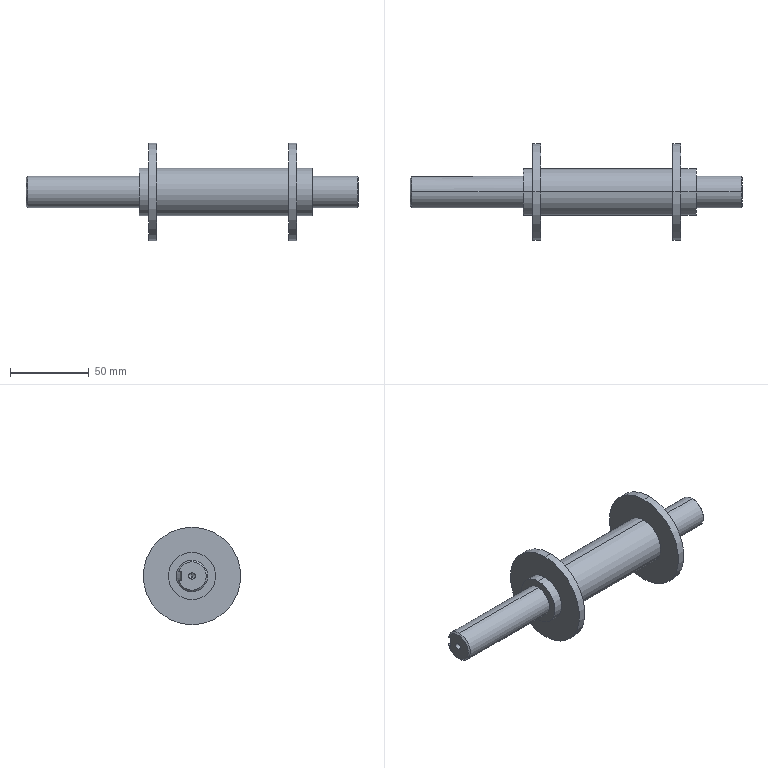Part | SolidWorks | features BaseBody 1 | 1 solid | 39 faces | box 211 x 62 x 62 mm | volume 131438 mm3 | cylinder 18 | plane 11 | cone 9 | spline 1 | commonest cylinder face diameters 30 x6 4.2 x4 20 x4 62 x4
STEP:
#1=CARTESIAN_POINT('',(73.6,0.,2.1));
#2=VERTEX_POINT('',#1);
#3=CARTESIAN_POINT('',(73.6,0.,-2.1));
#4=VERTEX_POINT('',#3);
#5=CARTESIAN_POINT('',(73.6,0.,0.));
#6=DIRECTION('',(1.,0.,0.));
#7=DIRECTION('',(0.,0.,-1.));
#8=AXIS2_PLACEMENT_3D('',#5,#6,#7);
#9=CIRCLE('',#8,2.1);
#10=EDGE_CURVE('',#2,#4,#9,.T.);
#11=ORIENTED_EDGE('',*,*,#10,.F.);
#12=CARTESIAN_POINT('',(86.,0.,2.1));
#13=VERTEX_POINT('',#12);
#14=CARTESIAN_POINT('',(86.,0.,2.1));
#15=DIRECTION('',(1.,0.,0.));
#16=VECTOR('',#15,1000.);
#17=LINE('',#14,#16);
#18=EDGE_CURVE('',#2,#13,#17,.T.);
#19=ORIENTED_EDGE('',*,*,#18,.T.);
#20=CARTESIAN_POINT('',(86.,0.,-2.1));
#21=VERTEX_POINT('',#20);
#22=CARTESIAN_POINT('',(86.,0.,0.));
#23=DIRECTION('',(1.,0.,0.));
#24=DIRECTION('',(0.,0.,-1.));
#25=AXIS2_PLACEMENT_3D('',#22,#23,#24);
#26=CIRCLE('',#25,2.1);
#27=EDGE_CURVE('',#13,#21,#26,.T.);
#28=ORIENTED_EDGE('',*,*,#27,.T.);
#29=CARTESIAN_POINT('',(86.,0.,-2.1));
#30=DIRECTION('',(1.,0.,0.));
#31=VECTOR('',#30,1000.);
#32=LINE('',#29,#31);
#33=EDGE_CURVE('',#4,#21,#32,.T.);
#34=ORIENTED_EDGE('',*,*,#33,.F.);
#35=EDGE_LOOP('',(#11,#19,#28,#34));
#36=FACE_OUTER_BOUND('',#35,.T.);
#37=CARTESIAN_POINT('',(86.,0.,0.));
#38=DIRECTION('',(1.,0.,0.));
#39=DIRECTION('',(0.,0.,-1.));
#40=AXIS2_PLACEMENT_3D('',#37,#38,#39);
#41=CYLINDRICAL_SURFACE('',#40,2.1);
#42=ADVANCED_FACE('',(#36),#41,.F.);
#43=CARTESIAN_POINT('',(72.338,0.,0.));
#44=VERTEX_POINT('',#43);
#45=CARTESIAN_POINT('',(73.6,0.,-2.1));
#46=DIRECTION('',(0.515,0.,-0.8572));
#47=VECTOR('',#46,1000.);
#48=LINE('',#45,#47);
#49=EDGE_CURVE('',#44,#4,#48,.T.);
#50=ORIENTED_EDGE('',*,*,#49,.F.);
#51=CARTESIAN_POINT('',(73.6,0.,2.1));
#52=DIRECTION('',(0.515,0.,0.8572));
#53=VECTOR('',#52,1000.);
#54=LINE('',#51,#53);
#55=EDGE_CURVE('',#44,#2,#54,.T.);
#56=ORIENTED_EDGE('',*,*,#55,.T.);
#57=ORIENTED_EDGE('',*,*,#10,.T.);
#58=EDGE_LOOP('',(#50,#56,#57));
#59=FACE_OUTER_BOUND('',#58,.T.);
#60=CARTESIAN_POINT('',(73.6,0.,0.));
#61=DIRECTION('',(1.,0.,0.));
#62=DIRECTION('',(0.,0.,-1.));
#63=AXIS2_PLACEMENT_3D('',#60,#61,#62);
#64=CONICAL_SURFACE('',#63,2.1,1.03);
#65=ADVANCED_FACE('',(#59),#64,.F.);
#66=CARTESIAN_POINT('',(-112.6,0.,-2.1));
#67=VERTEX_POINT('',#66);
#68=CARTESIAN_POINT('',(-112.6,0.,2.1));
#69=VERTEX_POINT('',#68);
#70=CARTESIAN_POINT('',(-112.6,0.,0.));
#71=DIRECTION('',(-1.,0.,0.));
#72=DIRECTION('',(0.,0.,1.));
#73=AXIS2_PLACEMENT_3D('',#70,#71,#72);
#74=CIRCLE('',#73,2.1);
#75=EDGE_CURVE('',#67,#69,#74,.T.);
#76=ORIENTED_EDGE('',*,*,#75,.F.);
#77=CARTESIAN_POINT('',(-125.,0.,-2.1));
#78=VERTEX_POINT('',#77);
#79=CARTESIAN_POINT('',(-125.,0.,-2.1));
#80=DIRECTION('',(-1.,0.,0.));
#81=VECTOR('',#80,1000.);
#82=LINE('',#79,#81);
#83=EDGE_CURVE('',#67,#78,#82,.T.);
#84=ORIENTED_EDGE('',*,*,#83,.T.);
#85=CARTESIAN_POINT('',(-125.,0.,2.1));
#86=VERTEX_POINT('',#85);
#87=CARTESIAN_POINT('',(-125.,0.,0.));
#88=DIRECTION('',(-1.,0.,0.));
#89=DIRECTION('',(0.,0.,1.));
#90=AXIS2_PLACEMENT_3D('',#87,#88,#89);
#91=CIRCLE('',#90,2.1);
#92=EDGE_CURVE('',#78,#86,#91,.T.);
#93=ORIENTED_EDGE('',*,*,#92,.T.);
#94=CARTESIAN_POINT('',(-125.,0.,2.1));
#95=DIRECTION('',(-1.,0.,0.));
#96=VECTOR('',#95,1000.);
#97=LINE('',#94,#96);
#98=EDGE_CURVE('',#69,#86,#97,.T.);
#99=ORIENTED_EDGE('',*,*,#98,.F.);
#100=EDGE_LOOP('',(#76,#84,#93,#99));
#101=FACE_OUTER_BOUND('',#100,.T.);
#102=CARTESIAN_POINT('',(-125.,0.,0.));
#103=DIRECTION('',(-1.,0.,0.));
#104=DIRECTION('',(0.,0.,1.));
#105=AXIS2_PLACEMENT_3D('',#102,#103,#104);
#106=CYLINDRICAL_SURFACE('',#105,2.1);
#107=ADVANCED_FACE('',(#101),#106,.F.);
#108=CARTESIAN_POINT('',(-111.338,0.,0.));
#109=VERTEX_POINT('',#108);
#110=CARTESIAN_POINT('',(-112.6,0.,2.1));
#111=DIRECTION('',(-0.515,0.,0.8572));
#112=VECTOR('',#111,1000.);
#113=LINE('',#110,#112);
#114=EDGE_CURVE('',#109,#69,#113,.T.);
#115=ORIENTED_EDGE('',*,*,#114,.F.);
#116=CARTESIAN_POINT('',(-112.6,0.,-2.1));
#117=DIRECTION('',(-0.515,0.,-0.8572));
#118=VECTOR('',#117,1000.);
#119=LINE('',#116,#118);
#120=EDGE_CURVE('',#109,#67,#119,.T.);
#121=ORIENTED_EDGE('',*,*,#120,.T.);
#122=ORIENTED_EDGE('',*,*,#75,.T.);
#123=EDGE_LOOP('',(#115,#121,#122));
#124=FACE_OUTER_BOUND('',#123,.T.);
#125=CARTESIAN_POINT('',(-112.6,0.,0.));
#126=DIRECTION('',(-1.,0.,0.));
#127=DIRECTION('',(0.,0.,1.));
#128=AXIS2_PLACEMENT_3D('',#125,#126,#127);
#129=CONICAL_SURFACE('',#128,2.1,1.03);
#130=ADVANCED_FACE('',(#124),#129,.F.);
#131=CARTESIAN_POINT('',(86.,0.,-9.5));
#132=VERTEX_POINT('',#131);
#133=CARTESIAN_POINT('',(86.,0.,9.5));
#134=VERTEX_POINT('',#133);
#135=CARTESIAN_POINT('',(86.,0.,0.));
#136=DIRECTION('',(1.,0.,0.));
#137=DIRECTION('',(0.,0.,-1.));
#138=AXIS2_PLACEMENT_3D('',#135,#136,#137);
#139=CIRCLE('',#138,9.5);
#140=EDGE_CURVE('',#132,#134,#139,.T.);
#141=ORIENTED_EDGE('',*,*,#140,.F.);
#142=CARTESIAN_POINT('',(85.5,0.,-10.));
#143=VERTEX_POINT('',#142);
#144=CARTESIAN_POINT('',(86.,0.,-9.5));
#145=DIRECTION('',(-0.7071,0.,-0.7071));
#146=VECTOR('',#145,1000.);
#147=LINE('',#144,#146);
#148=EDGE_CURVE('',#132,#143,#147,.T.);
#149=ORIENTED_EDGE('',*,*,#148,.T.);
#150=CARTESIAN_POINT('',(85.5,0.,10.));
#151=VERTEX_POINT('',#150);
#152=CARTESIAN_POINT('',(85.5,0.,0.));
#153=DIRECTION('',(-1.,0.,0.));
#154=DIRECTION('',(0.,0.,-1.));
#155=AXIS2_PLACEMENT_3D('',#152,#153,#154);
#156=CIRCLE('',#155,10.);
#157=EDGE_CURVE('',#151,#143,#156,.T.);
#158=ORIENTED_EDGE('',*,*,#157,.F.);
#159=CARTESIAN_POINT('',(86.,0.,9.5));
#160=DIRECTION('',(-0.7071,0.,0.7071));
#161=VECTOR('',#160,1000.);
#162=LINE('',#159,#161);
#163=EDGE_CURVE('',#134,#151,#162,.T.);
#164=ORIENTED_EDGE('',*,*,#163,.F.);
#165=EDGE_LOOP('',(#141,#149,#158,#164));
#166=FACE_OUTER_BOUND('',#165,.T.);
#167=CARTESIAN_POINT('',(86.,0.,0.));
#168=DIRECTION('',(-1.,0.,0.));
#169=DIRECTION('',(0.,0.,1.));
#170=AXIS2_PLACEMENT_3D('',#167,#168,#169);
#171=CONICAL_SURFACE('',#170,9.5,0.7854);
#172=ADVANCED_FACE('',(#166),#171,.T.);
#173=ORIENTED_EDGE('',*,*,#157,.T.);
#174=CARTESIAN_POINT('',(57.,0.,-10.));
#175=VERTEX_POINT('',#174);
#176=CARTESIAN_POINT('',(86.,0.,-10.));
#177=DIRECTION('',(-1.,0.,0.));
#178=VECTOR('',#177,1000.);
#179=LINE('',#176,#178);
#180=EDGE_CURVE('',#143,#175,#179,.T.);
#181=ORIENTED_EDGE('',*,*,#180,.T.);
#182=CARTESIAN_POINT('',(57.,0.,10.));
#183=VERTEX_POINT('',#182);
#184=CARTESIAN_POINT('',(57.,0.,0.));
#185=DIRECTION('',(1.,0.,0.));
#186=DIRECTION('',(0.,0.,-1.));
#187=AXIS2_PLACEMENT_3D('',#184,#185,#186);
#188=CIRCLE('',#187,10.);
#189=EDGE_CURVE('',#175,#183,#188,.T.);
#190=ORIENTED_EDGE('',*,*,#189,.T.);
#191=CARTESIAN_POINT('',(86.,0.,10.));
#192=DIRECTION('',(-1.,0.,0.));
#193=VECTOR('',#192,1000.);
#194=LINE('',#191,#193);
#195=EDGE_CURVE('',#151,#183,#194,.T.);
#196=ORIENTED_EDGE('',*,*,#195,.F.);
#197=EDGE_LOOP('',(#173,#181,#190,#196));
#198=FACE_OUTER_BOUND('',#197,.T.);
#199=CARTESIAN_POINT('',(86.,0.,0.));
#200=DIRECTION('',(-1.,0.,0.));
#201=DIRECTION('',(0.,0.,1.));
#202=AXIS2_PLACEMENT_3D('',#199,#200,#201);
#203=CYLINDRICAL_SURFACE('',#202,10.);
#204=ADVANCED_FACE('',(#198),#203,.T.);
#205=CARTESIAN_POINT('',(-125.,0.,9.));
#206=VERTEX_POINT('',#205);
#207=CARTESIAN_POINT('',(-125.,8.485,3.));
#208=VERTEX_POINT('',#207);
#209=CARTESIAN_POINT('',(-125.,0.,0.));
#210=DIRECTION('',(-1.,0.,0.));
#211=DIRECTION('',(0.,0.,1.));
#212=AXIS2_PLACEMENT_3D('',#209,#210,#211);
#213=CIRCLE('',#212,9.);
#214=EDGE_CURVE('',#206,#208,#213,.T.);
#215=ORIENTED_EDGE('',*,*,#214,.F.);
#216=CARTESIAN_POINT('',(-124.,0.,10.));
#217=VERTEX_POINT('',#216);
#218=CARTESIAN_POINT('',(-125.,0.,9.));
#219=DIRECTION('',(0.7071,0.,0.7071));
#220=VECTOR('',#219,1000.);
#221=LINE('',#218,#220);
#222=EDGE_CURVE('',#206,#217,#221,.T.);
#223=ORIENTED_EDGE('',*,*,#222,.T.);
#224=CARTESIAN_POINT('',(-124.,9.539,3.));
#225=VERTEX_POINT('',#224);
#226=CARTESIAN_POINT('',(-124.,0.,0.));
#227=DIRECTION('',(1.,0.,0.));
#228=DIRECTION('',(0.,0.,1.));
#229=AXIS2_PLACEMENT_3D('',#226,#227,#228);
#230=CIRCLE('',#229,10.);
#231=EDGE_CURVE('',#225,#217,#230,.T.);
#232=ORIENTED_EDGE('',*,*,#231,.F.);
#233=CARTESIAN_POINT('',(-125.,8.485,3.));
#234=CARTESIAN_POINT('',(-124.668,8.838,3.));
#235=CARTESIAN_POINT('',(-124.334,9.189,3.));
#236=CARTESIAN_POINT('',(-124.,9.539,3.));
#237=B_SPLINE_CURVE_WITH_KNOTS('',3,(#233,#234,#235,#236),.UNSPECIFIED.,.F.,.F.,(4,4),(0.006491,0.007944),.UNSPECIFIED.);
#238=EDGE_CURVE('',#208,#225,#237,.T.);
#239=ORIENTED_EDGE('',*,*,#238,.F.);
#240=EDGE_LOOP('',(#215,#223,#232,#239));
#241=FACE_OUTER_BOUND('',#240,.T.);
#242=CARTESIAN_POINT('',(-125.,0.,0.));
#243=DIRECTION('',(1.,0.,0.));
#244=DIRECTION('',(0.,0.,-1.));
#245=AXIS2_PLACEMENT_3D('',#242,#243,#244);
#246=CONICAL_SURFACE('',#245,9.,0.7854);
#247=ADVANCED_FACE('',(#241),#246,.T.);
#248=ORIENTED_EDGE('',*,*,#222,.F.);
#249=CARTESIAN_POINT('',(-125.,0.,-9.));
#250=VERTEX_POINT('',#249);
#251=CARTESIAN_POINT('',(-125.,0.,0.));
#252=DIRECTION('',(-1.,0.,0.));
#253=DIRECTION('',(0.,0.,1.));
#254=AXIS2_PLACEMENT_3D('',#251,#252,#253);
#255=CIRCLE('',#254,9.);
#256=EDGE_CURVE('',#250,#206,#255,.T.);
#257=ORIENTED_EDGE('',*,*,#256,.F.);
#258=CARTESIAN_POINT('',(-124.,0.,-10.));
#259=VERTEX_POINT('',#258);
#260=CARTESIAN_POINT('',(-125.,0.,-9.));
#261=DIRECTION('',(0.7071,0.,-0.7071));
#262=VECTOR('',#261,1000.);
#263=LINE('',#260,#262);
#264=EDGE_CURVE('',#250,#259,#263,.T.);
#265=ORIENTED_EDGE('',*,*,#264,.T.);
#266=CARTESIAN_POINT('',(-124.,0.,0.));
#267=DIRECTION('',(1.,0.,0.));
#268=DIRECTION('',(0.,0.,1.));
#269=AXIS2_PLACEMENT_3D('',#266,#267,#268);
#270=CIRCLE('',#269,10.);
#271=EDGE_CURVE('',#217,#259,#270,.T.);
#272=ORIENTED_EDGE('',*,*,#271,.F.);
#273=EDGE_LOOP('',(#248,#257,#265,#272));
#274=FACE_OUTER_BOUND('',#273,.T.);
#275=CARTESIAN_POINT('',(-125.,0.,0.));
#276=DIRECTION('',(1.,0.,0.));
#277=DIRECTION('',(0.,0.,-1.));
#278=AXIS2_PLACEMENT_3D('',#275,#276,#277);
#279=CONICAL_SURFACE('',#278,9.,0.7854);
#280=ADVANCED_FACE('',(#274),#279,.T.);
#281=ORIENTED_EDGE('',*,*,#231,.T.);
#282=CARTESIAN_POINT('',(-53.,0.,10.));
#283=VERTEX_POINT('',#282);
#284=CARTESIAN_POINT('',(-125.,0.,10.));
#285=DIRECTION('',(1.,0.,0.));
#286=VECTOR('',#285,1000.);
#287=LINE('',#284,#286);
#288=EDGE_CURVE('',#217,#283,#287,.T.);
#289=ORIENTED_EDGE('',*,*,#288,.T.);
#290=CARTESIAN_POINT('',(-53.,0.,-10.));
#291=VERTEX_POINT('',#290);
#292=CARTESIAN_POINT('',(-53.,0.,0.));
#293=DIRECTION('',(-1.,0.,0.));
#294=DIRECTION('',(0.,0.,1.));
#295=AXIS2_PLACEMENT_3D('',#292,#293,#294);
#296=CIRCLE('',#295,10.);
#297=EDGE_CURVE('',#283,#291,#296,.T.);
#298=ORIENTED_EDGE('',*,*,#297,.T.);
#299=CARTESIAN_POINT('',(-125.,0.,-10.));
#300=DIRECTION('',(1.,0.,0.));
#301=VECTOR('',#300,1000.);
#302=LINE('',#299,#301);
#303=EDGE_CURVE('',#259,#291,#302,.T.);
#304=ORIENTED_EDGE('',*,*,#303,.F.);
#305=CARTESIAN_POINT('',(-124.,9.539,-3.));
#306=VERTEX_POINT('',#305);
#307=CARTESIAN_POINT('',(-124.,0.,0.));
#308=DIRECTION('',(1.,0.,0.));
#309=DIRECTION('',(0.,0.,1.));
#310=AXIS2_PLACEMENT_3D('',#307,#308,#309);
#311=CIRCLE('',#310,10.);
#312=EDGE_CURVE('',#259,#306,#311,.T.);
#313=ORIENTED_EDGE('',*,*,#312,.T.);
#314=CARTESIAN_POINT('',(-85.,9.539,-3.));
#315=VERTEX_POINT('',#314);
#316=CARTESIAN_POINT('',(-125.,9.539,-3.));
#317=DIRECTION('',(1.,0.,0.));
#318=VECTOR('',#317,1000.);
#319=LINE('',#316,#318);
#320=EDGE_CURVE('',#306,#315,#319,.T.);
#321=ORIENTED_EDGE('',*,*,#320,.T.);
#322=CARTESIAN_POINT('',(-85.,9.539,3.));
#323=VERTEX_POINT('',#322);
#324=CARTESIAN_POINT('',(-85.,9.539,3.));
#325=CARTESIAN_POINT('',(-85.,9.692,2.514));
#326=CARTESIAN_POINT('',(-85.,9.807,2.019));
#327=CARTESIAN_POINT('',(-85.,9.962,1.011));
#328=CARTESIAN_POINT('',(-85.,10.,0.5036));
#329=CARTESIAN_POINT('',(-85.,10.,-0.5143));
#330=CARTESIAN_POINT('',(-85.,9.96,-1.022));
#331=CARTESIAN_POINT('',(-85.,9.807,-2.021));
#332=CARTESIAN_POINT('',(-85.,9.692,-2.514));
#333=CARTESIAN_POINT('',(-85.,9.539,-3.));
#334=B_SPLINE_CURVE_WITH_KNOTS('',3,(#324,#325,#326,#327,#328,#329,#330,#331,#332,#333),.UNSPECIFIED.,.F.,.F.,(4,2,2,2,4),(0.,0.001525,0.003049,0.004574,0.006098),.UNSPECIFIED.);
#335=EDGE_CURVE('',#323,#315,#334,.T.);
#336=ORIENTED_EDGE('',*,*,#335,.F.);
#337=CARTESIAN_POINT('',(-125.,9.539,3.));
#338=DIRECTION('',(-1.,0.,0.));
#339=VECTOR('',#338,1000.);
#340=LINE('',#337,#339);
#341=EDGE_CURVE('',#323,#225,#340,.T.);
#342=ORIENTED_EDGE('',*,*,#341,.T.);
#343=EDGE_LOOP('',(#281,#289,#298,#304,#313,#321,#336,#342));
#344=FACE_OUTER_BOUND('',#343,.T.);
#345=CARTESIAN_POINT('',(-125.,0.,0.));
#346=DIRECTION('',(1.,0.,0.));
#347=DIRECTION('',(0.,0.,-1.));
#348=AXIS2_PLACEMENT_3D('',#345,#346,#347);
#349=CYLINDRICAL_SURFACE('',#348,10.);
#350=ADVANCED_FACE('',(#344),#349,.T.);
#351=CARTESIAN_POINT('',(57.,0.,15.));
#352=VERTEX_POINT('',#351);
#353=CARTESIAN_POINT('',(57.,0.,-15.));
#354=VERTEX_POINT('',#353);
#355=CARTESIAN_POINT('',(57.,0.,0.));
#356=DIRECTION('',(-1.,0.,0.));
#357=DIRECTION('',(0.,0.,1.));
#358=AXIS2_PLACEMENT_3D('',#355,#356,#357);
#359=CIRCLE('',#358,15.);
#360=EDGE_CURVE('',#352,#354,#359,.T.);
#361=ORIENTED_EDGE('',*,*,#360,.T.);
#362=CARTESIAN_POINT('',(47.,0.,-15.));
#363=VERTEX_POINT('',#362);
#364=CARTESIAN_POINT('',(-47.,0.,-15.));
#365=DIRECTION('',(-1.,0.,0.));
#366=VECTOR('',#365,1000.);
#367=LINE('',#364,#366);
#368=EDGE_CURVE('',#354,#363,#367,.T.);
#369=ORIENTED_EDGE('',*,*,#368,.T.);
#370=CARTESIAN_POINT('',(47.,0.,15.));
#371=VERTEX_POINT('',#370);
#372=CARTESIAN_POINT('',(47.,0.,0.));
#373=DIRECTION('',(-1.,0.,0.));
#374=DIRECTION('',(0.,0.,1.));
#375=AXIS2_PLACEMENT_3D('',#372,#373,#374);
#376=CIRCLE('',#375,15.);
#377=EDGE_CURVE('',#371,#363,#376,.T.);
#378=ORIENTED_EDGE('',*,*,#377,.F.);
#379=CARTESIAN_POINT('',(-47.,0.,15.));
#380=DIRECTION('',(-1.,0.,0.));
#381=VECTOR('',#380,1000.);
#382=LINE('',#379,#381);
#383=EDGE_CURVE('',#352,#371,#382,.T.);
#384=ORIENTED_EDGE('',*,*,#383,.F.);
#385=EDGE_LOOP('',(#361,#369,#378,#384));
#386=FACE_OUTER_BOUND('',#385,.T.);
#387=CARTESIAN_POINT('',(-47.,0.,0.));
#388=DIRECTION('',(-1.,0.,0.));
#389=DIRECTION('',(0.,0.,1.));
#390=AXIS2_PLACEMENT_3D('',#387,#388,#389);
#391=CYLINDRICAL_SURFACE('',#390,15.);
#392=ADVANCED_FACE('',(#386),#391,.T.);
#393=CARTESIAN_POINT('',(47.,0.,31.));
#394=VERTEX_POINT('',#393);
#395=CARTESIAN_POINT('',(47.,0.,-31.));
#396=VERTEX_POINT('',#395);
#397=CARTESIAN_POINT('',(47.,0.,0.));
#398=DIRECTION('',(-1.,0.,0.));
#399=DIRECTION('',(0.,0.,1.));
#400=AXIS2_PLACEMENT_3D('',#397,#398,#399);
#401=CIRCLE('',#400,31.);
#402=EDGE_CURVE('',#394,#396,#401,.T.);
#403=ORIENTED_EDGE('',*,*,#402,.T.);
#404=CARTESIAN_POINT('',(42.,0.,-31.));
#405=VERTEX_POINT('',#404);
#406=CARTESIAN_POINT('',(-47.,0.,-31.));
#407=DIRECTION('',(-1.,0.,0.));
#408=VECTOR('',#407,1000.);
#409=LINE('',#406,#408);
#410=EDGE_CURVE('',#396,#405,#409,.T.);
#411=ORIENTED_EDGE('',*,*,#410,.T.);
#412=CARTESIAN_POINT('',(42.,0.,31.));
#413=VERTEX_POINT('',#412);
#414=CARTESIAN_POINT('',(42.,0.,0.));
#415=DIRECTION('',(1.,0.,0.));
#416=DIRECTION('',(0.,0.,-1.));
#417=AXIS2_PLACEMENT_3D('',#414,#415,#416);
#418=CIRCLE('',#417,31.);
#419=EDGE_CURVE('',#405,#413,#418,.T.);
#420=ORIENTED_EDGE('',*,*,#419,.T.);
#421=CARTESIAN_POINT('',(-47.,0.,31.));
#422=DIRECTION('',(-1.,0.,0.));
#423=VECTOR('',#422,1000.);
#424=LINE('',#421,#423);
#425=EDGE_CURVE('',#394,#413,#424,.T.);
#426=ORIENTED_EDGE('',*,*,#425,.F.);
#427=EDGE_LOOP('',(#403,#411,#420,#426));
#428=FACE_OUTER_BOUND('',#427,.T.);
#429=CARTESIAN_POINT('',(-47.,0.,0.));
#430=DIRECTION('',(-1.,0.,0.));
#431=DIRECTION('',(0.,0.,1.));
#432=AXIS2_PLACEMENT_3D('',#429,#430,#431);
#433=CYLINDRICAL_SURFACE('',#432,31.);
#434=ADVANCED_FACE('',(#428),#433,.T.);
#435=CARTESIAN_POINT('',(-47.,0.,15.));
#436=VERTEX_POINT('',#435);
#437=CARTESIAN_POINT('',(-47.,0.,-15.));
#438=VERTEX_POINT('',#437);
#439=CARTESIAN_POINT('',(-47.,0.,0.));
#440=DIRECTION('',(-1.,0.,0.));
#441=DIRECTION('',(0.,0.,-1.));
#442=AXIS2_PLACEMENT_3D('',#439,#440,#441);
#443=CIRCLE('',#442,15.);
#444=EDGE_CURVE('',#436,#438,#443,.T.);
#445=ORIENTED_EDGE('',*,*,#444,.T.);
#446=CARTESIAN_POINT('',(-53.,0.,-15.));
#447=VERTEX_POINT('',#446);
#448=CARTESIAN_POINT('',(-47.,0.,-15.));
#449=DIRECTION('',(-1.,0.,0.));
#450=VECTOR('',#449,1000.);
#451=LINE('',#448,#450);
#452=EDGE_CURVE('',#438,#447,#451,.T.);
#453=ORIENTED_EDGE('',*,*,#452,.T.);
#454=CARTESIAN_POINT('',(-53.,0.,15.));
#455=VERTEX_POINT('',#454);
#456=CARTESIAN_POINT('',(-53.,0.,0.));
#457=DIRECTION('',(-1.,0.,0.));
#458=DIRECTION('',(0.,0.,1.));
#459=AXIS2_PLACEMENT_3D('',#456,#457,#458);
#460=CIRCLE('',#459,15.);
#461=EDGE_CURVE('',#455,#447,#460,.T.);
#462=ORIENTED_EDGE('',*,*,#461,.F.);
#463=CARTESIAN_POINT('',(-47.,0.,15.));
#464=DIRECTION('',(-1.,0.,0.));
#465=VECTOR('',#464,1000.);
#466=LINE('',#463,#465);
#467=EDGE_CURVE('',#436,#455,#466,.T.);
#468=ORIENTED_EDGE('',*,*,#467,.F.);
#469=EDGE_LOOP('',(#445,#453,#462,#468));
#470=FACE_OUTER_BOUND('',#469,.T.);
#471=CARTESIAN_POINT('',(-47.,0.,0.));
#472=DIRECTION('',(-1.,0.,0.));
#473=DIRECTION('',(0.,0.,1.));
#474=AXIS2_PLACEMENT_3D('',#471,#472,#473);
#475=CYLINDRICAL_SURFACE('',#474,15.);
#476=ADVANCED_FACE('',(#470),#475,.T.);
#477=CARTESIAN_POINT('',(-42.,0.,-31.));
#478=VERTEX_POINT('',#477);
#479=CARTESIAN_POINT('',(-42.,0.,31.));
#480=VERTEX_POINT('',#479);
#481=CARTESIAN_POINT('',(-42.,0.,0.));
#482=DIRECTION('',(1.,0.,0.));
#483=DIRECTION('',(0.,0.,-1.));
#484=AXIS2_PLACEMENT_3D('',#481,#482,#483);
#485=CIRCLE('',#484,31.);
#486=EDGE_CURVE('',#478,#480,#485,.T.);
#487=ORIENTED_EDGE('',*,*,#486,.F.);
#488=CARTESIAN_POINT('',(-47.,0.,-31.));
#489=VERTEX_POINT('',#488);
#490=CARTESIAN_POINT('',(-47.,0.,-31.));
#491=DIRECTION('',(-1.,0.,0.));
#492=VECTOR('',#491,1000.);
#493=LINE('',#490,#492);
#494=EDGE_CURVE('',#478,#489,#493,.T.);
#495=ORIENTED_EDGE('',*,*,#494,.T.);
#496=CARTESIAN_POINT('',(-47.,0.,31.));
#497=VERTEX_POINT('',#496);
#498=CARTESIAN_POINT('',(-47.,0.,0.));
#499=DIRECTION('',(-1.,0.,0.));
#500=DIRECTION('',(0.,0.,1.));
#501=AXIS2_PLACEMENT_3D('',#498,#499,#500);
#502=CIRCLE('',#501,31.);
#503=EDGE_CURVE('',#497,#489,#502,.T.);
#504=ORIENTED_EDGE('',*,*,#503,.F.);
#505=CARTESIAN_POINT('',(-47.,0.,31.));
#506=DIRECTION('',(-1.,0.,0.));
#507=VECTOR('',#506,1000.);
#508=LINE('',#505,#507);
#509=EDGE_CURVE('',#480,#497,#508,.T.);
#510=ORIENTED_EDGE('',*,*,#509,.F.);
#511=EDGE_LOOP('',(#487,#495,#504,#510));
#512=FACE_OUTER_BOUND('',#511,.T.);
#513=CARTESIAN_POINT('',(-47.,0.,0.));
#514=DIRECTION('',(-1.,0.,0.));
#515=DIRECTION('',(0.,0.,1.));
#516=AXIS2_PLACEMENT_3D('',#513,#514,#515);
#517=CYLINDRICAL_SURFACE('',#516,31.);
#518=ADVANCED_FACE('',(#512),#517,.T.);
#519=CARTESIAN_POINT('',(42.,0.,-15.));
#520=VERTEX_POINT('',#519);
#521=CARTESIAN_POINT('',(42.,0.,15.));
#522=VERTEX_POINT('',#521);
#523=CARTESIAN_POINT('',(42.,0.,0.));
#524=DIRECTION('',(1.,0.,0.));
#525=DIRECTION('',(0.,0.,-1.));
#526=AXIS2_PLACEMENT_3D('',#523,#524,#525);
#527=CIRCLE('',#526,15.);
#528=EDGE_CURVE('',#520,#522,#527,.T.);
#529=ORIENTED_EDGE('',*,*,#528,.F.);
#530=CARTESIAN_POINT('',(-42.,0.,-15.));
#531=VERTEX_POINT('',#530);
#532=CARTESIAN_POINT('',(-47.,0.,-15.));
#533=DIRECTION('',(-1.,0.,0.));
#534=VECTOR('',#533,1000.);
#535=LINE('',#532,#534);
#536=EDGE_CURVE('',#520,#531,#535,.T.);
#537=ORIENTED_EDGE('',*,*,#536,.T.);
#538=CARTESIAN_POINT('',(-42.,0.,15.));
#539=VERTEX_POINT('',#538);
#540=CARTESIAN_POINT('',(-42.,0.,0.));
#541=DIRECTION('',(1.,0.,0.));
#542=DIRECTION('',(0.,0.,-1.));
#543=AXIS2_PLACEMENT_3D('',#540,#541,#542);
#544=CIRCLE('',#543,15.);
#545=EDGE_CURVE('',#531,#539,#544,.T.);
#546=ORIENTED_EDGE('',*,*,#545,.T.);
#547=CARTESIAN_POINT('',(-47.,0.,15.));
#548=DIRECTION('',(-1.,0.,0.));
#549=VECTOR('',#548,1000.);
#550=LINE('',#547,#549);
#551=EDGE_CURVE('',#522,#539,#550,.T.);
#552=ORIENTED_EDGE('',*,*,#551,.F.);
#553=EDGE_LOOP('',(#529,#537,#546,#552));
#554=FACE_OUTER_BOUND('',#553,.T.);
#555=CARTESIAN_POINT('',(-47.,0.,0.));
#556=DIRECTION('',(-1.,0.,0.));
#557=DIRECTION('',(0.,0.,1.));
#558=AXIS2_PLACEMENT_3D('',#555,#556,#557);
#559=CYLINDRICAL_SURFACE('',#558,15.);
#560=ADVANCED_FACE('',(#554),#559,.T.);
#561=CARTESIAN_POINT('',(-89.631,6.5,-3.));
#562=VERTEX_POINT('',#561);
#563=CARTESIAN_POINT('',(-89.631,6.5,-3.));
#564=CARTESIAN_POINT('',(-89.138,6.5,-3.));
#565=CARTESIAN_POINT('',(-88.657,6.571,-3.));
#566=CARTESIAN_POINT('',(-87.954,6.78,-3.));
#567=CARTESIAN_POINT('',(-87.722,6.868,-3.));
#568=CARTESIAN_POINT('',(-87.28,7.073,-3.));
#569=CARTESIAN_POINT('',(-87.068,7.191,-3.));
#570=CARTESIAN_POINT('',(-86.66,7.458,-3.));
#571=CARTESIAN_POINT('',(-86.463,7.608,-3.));
#572=CARTESIAN_POINT('',(-86.097,7.933,-3.));
#573=CARTESIAN_POINT('',(-85.927,8.107,-3.));
#574=CARTESIAN_POINT('',(-85.457,8.664,-3.));
#575=CARTESIAN_POINT('',(-85.195,9.087,-3.));
#576=CARTESIAN_POINT('',(-85.,9.539,-3.));
#577=B_SPLINE_CURVE_WITH_KNOTS('',3,(#563,#564,#565,#566,#567,#568,#569,#570,#571,#572,#573,#574,#575,#576),.UNSPECIFIED.,.F.,.F.,(4,2,2,2,2,2,4),(0.,0.001458,0.002187,0.002916,0.003645,0.004373,0.005831),.UNSPECIFIED.);
#578=EDGE_CURVE('',#562,#315,#577,.T.);
#579=ORIENTED_EDGE('',*,*,#578,.F.);
#580=CARTESIAN_POINT('',(-89.631,6.5,3.));
#581=VERTEX_POINT('',#580);
#582=CARTESIAN_POINT('',(-89.631,6.5,3.));
#583=CARTESIAN_POINT('',(-89.734,6.5,2.002));
#584=CARTESIAN_POINT('',(-89.77,6.5,0.9991));
#585=CARTESIAN_POINT('',(-89.77,6.5,-1.002));
#586=CARTESIAN_POINT('',(-89.734,6.5,-2.002));
#587=CARTESIAN_POINT('',(-89.631,6.5,-3.));
#588=B_SPLINE_CURVE_WITH_KNOTS('',3,(#582,#583,#584,#585,#586,#587),.UNSPECIFIED.,.F.,.F.,(4,2,4),(0.,0.003008,0.006016),.UNSPECIFIED.);
#589=EDGE_CURVE('',#581,#562,#588,.T.);
#590=ORIENTED_EDGE('',*,*,#589,.F.);
#591=CARTESIAN_POINT('',(-85.,9.539,3.));
#592=CARTESIAN_POINT('',(-85.195,9.087,3.));
#593=CARTESIAN_POINT('',(-85.451,8.673,3.));
#594=CARTESIAN_POINT('',(-85.923,8.111,3.));
#595=CARTESIAN_POINT('',(-86.096,7.934,3.));
#596=CARTESIAN_POINT('',(-86.46,7.611,3.));
#597=CARTESIAN_POINT('',(-86.653,7.463,3.));
#598=CARTESIAN_POINT('',(-87.061,7.195,3.));
#599=CARTESIAN_POINT('',(-87.277,7.075,3.));
#600=CARTESIAN_POINT('',(-87.72,6.869,3.));
#601=CARTESIAN_POINT('',(-87.948,6.782,3.));
#602=CARTESIAN_POINT('',(-88.646,6.573,3.));
#603=CARTESIAN_POINT('',(-89.138,6.5,3.));
#604=CARTESIAN_POINT('',(-89.631,6.5,3.));
#605=B_SPLINE_CURVE_WITH_KNOTS('',3,(#591,#592,#593,#594,#595,#596,#597,#598,#599,#600,#601,#602,#603,#604),.UNSPECIFIED.,.F.,.F.,(4,2,2,2,2,2,4),(0.,0.001458,0.002187,0.002915,0.003644,0.004373,0.005831),.UNSPECIFIED.);
#606=EDGE_CURVE('',#323,#581,#605,.T.);
#607=ORIENTED_EDGE('',*,*,#606,.F.);
#608=ORIENTED_EDGE('',*,*,#335,.T.);
#609=EDGE_LOOP('',(#579,#590,#607,#608));
#610=FACE_OUTER_BOUND('',#609,.T.);
#611=CARTESIAN_POINT('',(-85.,9.529,-3.032));
#612=CARTESIAN_POINT('',(-86.287,6.5,-3.21));
#613=CARTESIAN_POINT('',(-89.552,6.5,-3.66));
#614=CARTESIAN_POINT('',(-85.,9.674,-2.577));
#615=CARTESIAN_POINT('',(-86.242,6.5,-2.697));
#616=CARTESIAN_POINT('',(-89.636,6.5,-3.054));
#617=CARTESIAN_POINT('',(-85.,9.793,-2.088));
#618=CARTESIAN_POINT('',(-86.194,6.5,-2.175));
#619=CARTESIAN_POINT('',(-89.688,6.5,-2.447));
#620=CARTESIAN_POINT('',(-85.,9.956,-1.069));
#621=CARTESIAN_POINT('',(-86.122,6.5,-1.102));
#622=CARTESIAN_POINT('',(-89.755,6.5,-1.229));
#623=CARTESIAN_POINT('',(-85.,10.,-0.5385));
#624=CARTESIAN_POINT('',(-86.101,6.5,-0.5571));
#625=CARTESIAN_POINT('',(-89.77,6.5,-0.6192));
#626=CARTESIAN_POINT('',(-85.,10.,0.5242));
#627=CARTESIAN_POINT('',(-86.101,6.5,0.5423));
#628=CARTESIAN_POINT('',(-89.77,6.5,0.6028));
#629=CARTESIAN_POINT('',(-85.,9.958,1.056));
#630=CARTESIAN_POINT('',(-86.122,6.5,1.089));
#631=CARTESIAN_POINT('',(-89.755,6.5,1.215));
#632=CARTESIAN_POINT('',(-85.,9.794,2.084));
#633=CARTESIAN_POINT('',(-86.193,6.5,2.17));
#634=CARTESIAN_POINT('',(-89.688,6.5,2.441));
#635=CARTESIAN_POINT('',(-85.,9.674,2.576));
#636=CARTESIAN_POINT('',(-86.242,6.5,2.696));
#637=CARTESIAN_POINT('',(-89.636,6.5,3.052));
#638=CARTESIAN_POINT('',(-85.,9.529,3.033));
#639=CARTESIAN_POINT('',(-86.287,6.5,3.21));
#640=CARTESIAN_POINT('',(-89.552,6.5,3.66));
#641=(BOUNDED_SURFACE()B_SPLINE_SURFACE(3,2,((#611,#612,#613),(#614,#615,#616),(#617,#618,#619),(#620,#621,#622),(#623,#624,#625),(#626,#627,#628),(#629,#630,#631),(#632,#633,#634),(#635,#636,#637),(#638,#639,#640)),.UNSPECIFIED.,.F.,.F.,.T.)B_SPLINE_SURFACE_WITH_KNOTS((4,2,2,2,4),(3,3),(0.008171,0.01002,0.01187,0.01371,0.01556),(0.,1.),.UNSPECIFIED.)GEOMETRIC_REPRESENTATION_ITEM()RATIONAL_B_SPLINE_SURFACE(((1.,0.8349,1.),(1.,0.8262,1.),(1.,0.819,1.),(1.,0.809,1.),(1.,0.8062,1.),(1.,0.8062,1.),(1.,0.8089,1.),(1.,0.8189,1.),(1.,0.8262,1.),(1.,0.8349,1.)))REPRESENTATION_ITEM('')SURFACE());
#642=ADVANCED_FACE('',(#610),#641,.F.);
#643=CARTESIAN_POINT('',(-125.,6.5,3.));
#644=VERTEX_POINT('',#643);
#645=CARTESIAN_POINT('',(-85.,6.5,3.));
#646=DIRECTION('',(-1.,0.,0.));
#647=VECTOR('',#646,1000.);
#648=LINE('',#645,#647);
#649=EDGE_CURVE('',#581,#644,#648,.T.);
#650=ORIENTED_EDGE('',*,*,#649,.F.);
#651=ORIENTED_EDGE('',*,*,#589,.T.);
#652=CARTESIAN_POINT('',(-125.,6.5,-3.));
#653=VERTEX_POINT('',#652);
#654=CARTESIAN_POINT('',(-85.,6.5,-3.));
#655=DIRECTION('',(-1.,0.,0.));
#656=VECTOR('',#655,1000.);
#657=LINE('',#654,#656);
#658=EDGE_CURVE('',#562,#653,#657,.T.);
#659=ORIENTED_EDGE('',*,*,#658,.T.);
#660=CARTESIAN_POINT('',(-125.,6.5,-3.));
#661=DIRECTION('',(0.,0.,1.));
#662=VECTOR('',#661,1000.);
#663=LINE('',#660,#662);
#664=EDGE_CURVE('',#653,#644,#663,.T.);
#665=ORIENTED_EDGE('',*,*,#664,.T.);
#666=EDGE_LOOP('',(#650,#651,#659,#665));
#667=FACE_OUTER_BOUND('',#666,.T.);
#668=CARTESIAN_POINT('',(-85.,6.5,-3.));
#669=DIRECTION('',(0.,-1.,0.));
#670=DIRECTION('',(0.,0.,-1.));
#671=AXIS2_PLACEMENT_3D('',#668,#669,#670);
#672=PLANE('',#671);
#673=ADVANCED_FACE('',(#667),#672,.F.);
#674=ORIENTED_EDGE('',*,*,#341,.F.);
#675=ORIENTED_EDGE('',*,*,#606,.T.);
#676=ORIENTED_EDGE('',*,*,#649,.T.);
#677=CARTESIAN_POINT('',(-125.,12.8,3.));
#678=DIRECTION('',(0.,1.,0.));
#679=VECTOR('',#678,1000.);
#680=LINE('',#677,#679);
#681=EDGE_CURVE('',#644,#208,#680,.T.);
#682=ORIENTED_EDGE('',*,*,#681,.T.);
#683=ORIENTED_EDGE('',*,*,#238,.T.);
#684=EDGE_LOOP('',(#674,#675,#676,#682,#683));
#685=FACE_OUTER_BOUND('',#684,.T.);
#686=CARTESIAN_POINT('',(-85.,12.8,3.));
#687=DIRECTION('',(0.,0.,1.));
#688=DIRECTION('',(1.,0.,0.));
#689=AXIS2_PLACEMENT_3D('',#686,#687,#688);
#690=PLANE('',#689);
#691=ADVANCED_FACE('',(#685),#690,.F.);
#692=ORIENTED_EDGE('',*,*,#658,.F.);
#693=ORIENTED_EDGE('',*,*,#578,.T.);
#694=ORIENTED_EDGE('',*,*,#320,.F.);
#695=CARTESIAN_POINT('',(-125.,8.485,-3.));
#696=VERTEX_POINT('',#695);
#697=CARTESIAN_POINT('',(-124.,9.539,-3.));
#698=CARTESIAN_POINT('',(-124.334,9.189,-3.));
#699=CARTESIAN_POINT('',(-124.668,8.838,-3.));
#700=CARTESIAN_POINT('',(-125.,8.485,-3.));
#701=B_SPLINE_CURVE_WITH_KNOTS('',3,(#697,#698,#699,#700),.UNSPECIFIED.,.F.,.F.,(4,4),(0.006016,0.007469),.UNSPECIFIED.);
#702=EDGE_CURVE('',#306,#696,#701,.T.);
#703=ORIENTED_EDGE('',*,*,#702,.T.);
#704=CARTESIAN_POINT('',(-125.,12.8,-3.));
#705=DIRECTION('',(0.,-1.,0.));
#706=VECTOR('',#705,1000.);
#707=LINE('',#704,#706);
#708=EDGE_CURVE('',#696,#653,#707,.T.);
#709=ORIENTED_EDGE('',*,*,#708,.T.);
#710=EDGE_LOOP('',(#692,#693,#694,#703,#709));
#711=FACE_OUTER_BOUND('',#710,.T.);
#712=CARTESIAN_POINT('',(-85.,12.8,-3.));
#713=DIRECTION('',(0.,0.,-1.));
#714=DIRECTION('',(0.,-1.,0.));
#715=AXIS2_PLACEMENT_3D('',#712,#713,#714);
#716=PLANE('',#715);
#717=ADVANCED_FACE('',(#711),#716,.F.);
#718=CARTESIAN_POINT('',(86.,0.,0.));
#719=DIRECTION('',(1.,0.,0.));
#720=DIRECTION('',(0.,0.,-1.));
#721=AXIS2_PLACEMENT_3D('',#718,#719,#720);
#722=CIRCLE('',#721,2.1);
#723=EDGE_CURVE('',#21,#13,#722,.T.);
#724=ORIENTED_EDGE('',*,*,#723,.F.);
#725=ORIENTED_EDGE('',*,*,#27,.F.);
#726=EDGE_LOOP('',(#724,#725));
#727=FACE_BOUND('',#726,.T.);
#728=CARTESIAN_POINT('',(86.,0.,0.));
#729=DIRECTION('',(1.,0.,0.));
#730=DIRECTION('',(0.,0.,-1.));
#731=AXIS2_PLACEMENT_3D('',#728,#729,#730);
#732=CIRCLE('',#731,9.5);
#733=EDGE_CURVE('',#134,#132,#732,.T.);
#734=ORIENTED_EDGE('',*,*,#733,.T.);
#735=ORIENTED_EDGE('',*,*,#140,.T.);
#736=EDGE_LOOP('',(#734,#735));
#737=FACE_OUTER_BOUND('',#736,.T.);
#738=CARTESIAN_POINT('',(86.,0.,0.));
#739=DIRECTION('',(1.,0.,0.));
#740=DIRECTION('',(0.,1.,0.));
#741=AXIS2_PLACEMENT_3D('',#738,#739,#740);
#742=PLANE('',#741);
#743=ADVANCED_FACE('',(#727,#737),#742,.T.);
#744=CARTESIAN_POINT('',(-125.,0.,0.));
#745=DIRECTION('',(-1.,0.,0.));
#746=DIRECTION('',(0.,0.,1.));
#747=AXIS2_PLACEMENT_3D('',#744,#745,#746);
#748=CIRCLE('',#747,2.1);
#749=EDGE_CURVE('',#86,#78,#748,.T.);
#750=ORIENTED_EDGE('',*,*,#749,.F.);
#751=ORIENTED_EDGE('',*,*,#92,.F.);
#752=EDGE_LOOP('',(#750,#751));
#753=FACE_BOUND('',#752,.T.);
#754=ORIENTED_EDGE('',*,*,#708,.F.);
#755=CARTESIAN_POINT('',(-125.,0.,0.));
#756=DIRECTION('',(-1.,0.,0.));
#757=DIRECTION('',(0.,0.,1.));
#758=AXIS2_PLACEMENT_3D('',#755,#756,#757);
#759=CIRCLE('',#758,9.);
#760=EDGE_CURVE('',#696,#250,#759,.T.);
#761=ORIENTED_EDGE('',*,*,#760,.T.);
#762=ORIENTED_EDGE('',*,*,#256,.T.);
#763=ORIENTED_EDGE('',*,*,#214,.T.);
#764=ORIENTED_EDGE('',*,*,#681,.F.);
#765=ORIENTED_EDGE('',*,*,#664,.F.);
#766=EDGE_LOOP('',(#754,#761,#762,#763,#764,#765));
#767=FACE_OUTER_BOUND('',#766,.T.);
#768=CARTESIAN_POINT('',(-125.,0.,0.));
#769=DIRECTION('',(-1.,0.,0.));
#770=DIRECTION('',(0.,0.,1.));
#771=AXIS2_PLACEMENT_3D('',#768,#769,#770);
#772=PLANE('',#771);
#773=ADVANCED_FACE('',(#753,#767),#772,.T.);
#774=CARTESIAN_POINT('',(57.,0.,0.));
#775=DIRECTION('',(1.,0.,0.));
#776=DIRECTION('',(0.,0.,-1.));
#777=AXIS2_PLACEMENT_3D('',#774,#775,#776);
#778=CIRCLE('',#777,10.);
#779=EDGE_CURVE('',#183,#175,#778,.T.);
#780=ORIENTED_EDGE('',*,*,#779,.F.);
#781=ORIENTED_EDGE('',*,*,#189,.F.);
#782=EDGE_LOOP('',(#780,#781));
#783=FACE_BOUND('',#782,.T.);
#784=ORIENTED_EDGE('',*,*,#360,.F.);
#785=CARTESIAN_POINT('',(57.,0.,0.));
#786=DIRECTION('',(-1.,0.,0.));
#787=DIRECTION('',(0.,0.,1.));
#788=AXIS2_PLACEMENT_3D('',#785,#786,#787);
#789=CIRCLE('',#788,15.);
#790=EDGE_CURVE('',#354,#352,#789,.T.);
#791=ORIENTED_EDGE('',*,*,#790,.F.);
#792=EDGE_LOOP('',(#784,#791));
#793=FACE_OUTER_BOUND('',#792,.T.);
#794=CARTESIAN_POINT('',(57.,0.,0.));
#795=DIRECTION('',(-1.,0.,0.));
#796=DIRECTION('',(0.,0.,1.));
#797=AXIS2_PLACEMENT_3D('',#794,#795,#796);
#798=PLANE('',#797);
#799=ADVANCED_FACE('',(#783,#793),#798,.F.);
#800=CARTESIAN_POINT('',(42.,0.,0.));
#801=DIRECTION('',(1.,0.,0.));
#802=DIRECTION('',(0.,0.,-1.));
#803=AXIS2_PLACEMENT_3D('',#800,#801,#802);
#804=CIRCLE('',#803,15.);
#805=EDGE_CURVE('',#522,#520,#804,.T.);
#806=ORIENTED_EDGE('',*,*,#805,.T.);
#807=ORIENTED_EDGE('',*,*,#528,.T.);
#808=EDGE_LOOP('',(#806,#807));
#809=FACE_BOUND('',#808,.T.);
#810=CARTESIAN_POINT('',(42.,0.,0.));
#811=DIRECTION('',(1.,0.,0.));
#812=DIRECTION('',(0.,0.,-1.));
#813=AXIS2_PLACEMENT_3D('',#810,#811,#812);
#814=CIRCLE('',#813,31.);
#815=EDGE_CURVE('',#413,#405,#814,.T.);
#816=ORIENTED_EDGE('',*,*,#815,.F.);
#817=ORIENTED_EDGE('',*,*,#419,.F.);
#818=EDGE_LOOP('',(#816,#817));
#819=FACE_OUTER_BOUND('',#818,.T.);
#820=CARTESIAN_POINT('',(42.,0.,0.));
#821=DIRECTION('',(1.,0.,0.));
#822=DIRECTION('',(0.,1.,0.));
#823=AXIS2_PLACEMENT_3D('',#820,#821,#822);
#824=PLANE('',#823);
#825=ADVANCED_FACE('',(#809,#819),#824,.F.);
#826=ORIENTED_EDGE('',*,*,#377,.T.);
#827=CARTESIAN_POINT('',(47.,0.,0.));
#828=DIRECTION('',(-1.,0.,0.));
#829=DIRECTION('',(0.,0.,1.));
#830=AXIS2_PLACEMENT_3D('',#827,#828,#829);
#831=CIRCLE('',#830,15.);
#832=EDGE_CURVE('',#363,#371,#831,.T.);
#833=ORIENTED_EDGE('',*,*,#832,.T.);
#834=EDGE_LOOP('',(#826,#833));
#835=FACE_BOUND('',#834,.T.);
#836=ORIENTED_EDGE('',*,*,#402,.F.);
#837=CARTESIAN_POINT('',(47.,0.,0.));
#838=DIRECTION('',(-1.,0.,0.));
#839=DIRECTION('',(0.,0.,1.));
#840=AXIS2_PLACEMENT_3D('',#837,#838,#839);
#841=CIRCLE('',#840,31.);
#842=EDGE_CURVE('',#396,#394,#841,.T.);
#843=ORIENTED_EDGE('',*,*,#842,.F.);
#844=EDGE_LOOP('',(#836,#843));
#845=FACE_OUTER_BOUND('',#844,.T.);
#846=CARTESIAN_POINT('',(47.,0.,0.));
#847=DIRECTION('',(-1.,0.,0.));
#848=DIRECTION('',(0.,0.,1.));
#849=AXIS2_PLACEMENT_3D('',#846,#847,#848);
#850=PLANE('',#849);
#851=ADVANCED_FACE('',(#835,#845),#850,.F.);
#852=CARTESIAN_POINT('',(-53.,0.,0.));
#853=DIRECTION('',(-1.,0.,0.));
#854=DIRECTION('',(0.,0.,1.));
#855=AXIS2_PLACEMENT_3D('',#852,#853,#854);
#856=CIRCLE('',#855,10.);
#857=EDGE_CURVE('',#291,#283,#856,.T.);
#858=ORIENTED_EDGE('',*,*,#857,.F.);
#859=ORIENTED_EDGE('',*,*,#297,.F.);
#860=EDGE_LOOP('',(#858,#859));
#861=FACE_BOUND('',#860,.T.);
#862=ORIENTED_EDGE('',*,*,#461,.T.);
#863=CARTESIAN_POINT('',(-53.,0.,0.));
#864=DIRECTION('',(-1.,0.,0.));
#865=DIRECTION('',(0.,0.,1.));
#866=AXIS2_PLACEMENT_3D('',#863,#864,#865);
#867=CIRCLE('',#866,15.);
#868=EDGE_CURVE('',#447,#455,#867,.T.);
#869=ORIENTED_EDGE('',*,*,#868,.T.);
#870=EDGE_LOOP('',(#862,#869));
#871=FACE_OUTER_BOUND('',#870,.T.);
#872=CARTESIAN_POINT('',(-53.,15.,0.));
#873=DIRECTION('',(1.,0.,0.));
#874=DIRECTION('',(0.,1.,0.));
#875=AXIS2_PLACEMENT_3D('',#872,#873,#874);
#876=PLANE('',#875);
#877=ADVANCED_FACE('',(#861,#871),#876,.F.);
#878=CARTESIAN_POINT('',(-42.,0.,0.));
#879=DIRECTION('',(1.,0.,0.));
#880=DIRECTION('',(0.,0.,-1.));
#881=AXIS2_PLACEMENT_3D('',#878,#879,#880);
#882=CIRCLE('',#881,15.);
#883=EDGE_CURVE('',#539,#531,#882,.T.);
#884=ORIENTED_EDGE('',*,*,#883,.F.);
#885=ORIENTED_EDGE('',*,*,#545,.F.);
#886=EDGE_LOOP('',(#884,#885));
#887=FACE_BOUND('',#886,.T.);
#888=CARTESIAN_POINT('',(-42.,0.,0.));
#889=DIRECTION('',(1.,0.,0.));
#890=DIRECTION('',(0.,0.,-1.));
#891=AXIS2_PLACEMENT_3D('',#888,#889,#890);
#892=CIRCLE('',#891,31.);
#893=EDGE_CURVE('',#480,#478,#892,.T.);
#894=ORIENTED_EDGE('',*,*,#893,.T.);
#895=ORIENTED_EDGE('',*,*,#486,.T.);
#896=EDGE_LOOP('',(#894,#895));
#897=FACE_OUTER_BOUND('',#896,.T.);
#898=CARTESIAN_POINT('',(-42.,0.,0.));
#899=DIRECTION('',(1.,0.,0.));
#900=DIRECTION('',(0.,1.,0.));
#901=AXIS2_PLACEMENT_3D('',#898,#899,#900);
#902=PLANE('',#901);
#903=ADVANCED_FACE('',(#887,#897),#902,.T.);
#904=ORIENTED_EDGE('',*,*,#444,.F.);
#905=CARTESIAN_POINT('',(-47.,0.,0.));
#906=DIRECTION('',(-1.,0.,0.));
#907=DIRECTION('',(0.,0.,-1.));
#908=AXIS2_PLACEMENT_3D('',#905,#906,#907);
#909=CIRCLE('',#908,15.);
#910=EDGE_CURVE('',#438,#436,#909,.T.);
#911=ORIENTED_EDGE('',*,*,#910,.F.);
#912=EDGE_LOOP('',(#904,#911));
#913=FACE_BOUND('',#912,.T.);
#914=ORIENTED_EDGE('',*,*,#503,.T.);
#915=CARTESIAN_POINT('',(-47.,0.,0.));
#916=DIRECTION('',(-1.,0.,0.));
#917=DIRECTION('',(0.,0.,1.));
#918=AXIS2_PLACEMENT_3D('',#915,#916,#917);
#919=CIRCLE('',#918,31.);
#920=EDGE_CURVE('',#489,#497,#919,.T.);
#921=ORIENTED_EDGE('',*,*,#920,.T.);
#922=EDGE_LOOP('',(#914,#921));
#923=FACE_OUTER_BOUND('',#922,.T.);
#924=CARTESIAN_POINT('',(-47.,0.,0.));
#925=DIRECTION('',(1.,0.,0.));
#926=DIRECTION('',(0.,1.,0.));
#927=AXIS2_PLACEMENT_3D('',#924,#925,#926);
#928=PLANE('',#927);
#929=ADVANCED_FACE('',(#913,#923),#928,.F.);
#930=ORIENTED_EDGE('',*,*,#536,.F.);
#931=ORIENTED_EDGE('',*,*,#805,.F.);
#932=ORIENTED_EDGE('',*,*,#551,.T.);
#933=ORIENTED_EDGE('',*,*,#883,.T.);
#934=EDGE_LOOP('',(#930,#931,#932,#933));
#935=FACE_OUTER_BOUND('',#934,.T.);
#936=CARTESIAN_POINT('',(-47.,0.,0.));
#937=DIRECTION('',(-1.,0.,0.));
#938=DIRECTION('',(0.,0.,1.));
#939=AXIS2_PLACEMENT_3D('',#936,#937,#938);
#940=CYLINDRICAL_SURFACE('',#939,15.);
#941=ADVANCED_FACE('',(#935),#940,.T.);
#942=ORIENTED_EDGE('',*,*,#494,.F.);
#943=ORIENTED_EDGE('',*,*,#893,.F.);
#944=ORIENTED_EDGE('',*,*,#509,.T.);
#945=ORIENTED_EDGE('',*,*,#920,.F.);
#946=EDGE_LOOP('',(#942,#943,#944,#945));
#947=FACE_OUTER_BOUND('',#946,.T.);
#948=CARTESIAN_POINT('',(-47.,0.,0.));
#949=DIRECTION('',(-1.,0.,0.));
#950=DIRECTION('',(0.,0.,1.));
#951=AXIS2_PLACEMENT_3D('',#948,#949,#950);
#952=CYLINDRICAL_SURFACE('',#951,31.);
#953=ADVANCED_FACE('',(#947),#952,.T.);
#954=ORIENTED_EDGE('',*,*,#452,.F.);
#955=ORIENTED_EDGE('',*,*,#910,.T.);
#956=ORIENTED_EDGE('',*,*,#467,.T.);
#957=ORIENTED_EDGE('',*,*,#868,.F.);
#958=EDGE_LOOP('',(#954,#955,#956,#957));
#959=FACE_OUTER_BOUND('',#958,.T.);
#960=CARTESIAN_POINT('',(-47.,0.,0.));
#961=DIRECTION('',(-1.,0.,0.));
#962=DIRECTION('',(0.,0.,1.));
#963=AXIS2_PLACEMENT_3D('',#960,#961,#962);
#964=CYLINDRICAL_SURFACE('',#963,15.);
#965=ADVANCED_FACE('',(#959),#964,.T.);
#966=ORIENTED_EDGE('',*,*,#410,.F.);
#967=ORIENTED_EDGE('',*,*,#842,.T.);
#968=ORIENTED_EDGE('',*,*,#425,.T.);
#969=ORIENTED_EDGE('',*,*,#815,.T.);
#970=EDGE_LOOP('',(#966,#967,#968,#969));
#971=FACE_OUTER_BOUND('',#970,.T.);
#972=CARTESIAN_POINT('',(-47.,0.,0.));
#973=DIRECTION('',(-1.,0.,0.));
#974=DIRECTION('',(0.,0.,1.));
#975=AXIS2_PLACEMENT_3D('',#972,#973,#974);
#976=CYLINDRICAL_SURFACE('',#975,31.);
#977=ADVANCED_FACE('',(#971),#976,.T.);
#978=ORIENTED_EDGE('',*,*,#368,.F.);
#979=ORIENTED_EDGE('',*,*,#790,.T.);
#980=ORIENTED_EDGE('',*,*,#383,.T.);
#981=ORIENTED_EDGE('',*,*,#832,.F.);
#982=EDGE_LOOP('',(#978,#979,#980,#981));
#983=FACE_OUTER_BOUND('',#982,.T.);
#984=CARTESIAN_POINT('',(-47.,0.,0.));
#985=DIRECTION('',(-1.,0.,0.));
#986=DIRECTION('',(0.,0.,1.));
#987=AXIS2_PLACEMENT_3D('',#984,#985,#986);
#988=CYLINDRICAL_SURFACE('',#987,15.);
#989=ADVANCED_FACE('',(#983),#988,.T.);
#990=ORIENTED_EDGE('',*,*,#288,.F.);
#991=ORIENTED_EDGE('',*,*,#271,.T.);
#992=ORIENTED_EDGE('',*,*,#303,.T.);
#993=ORIENTED_EDGE('',*,*,#857,.T.);
#994=EDGE_LOOP('',(#990,#991,#992,#993));
#995=FACE_OUTER_BOUND('',#994,.T.);
#996=CARTESIAN_POINT('',(-125.,0.,0.));
#997=DIRECTION('',(1.,0.,0.));
#998=DIRECTION('',(0.,0.,-1.));
#999=AXIS2_PLACEMENT_3D('',#996,#997,#998);
#1000=CYLINDRICAL_SURFACE('',#999,10.);
#1001=ADVANCED_FACE('',(#995),#1000,.T.);
#1002=ORIENTED_EDGE('',*,*,#264,.F.);
#1003=ORIENTED_EDGE('',*,*,#760,.F.);
#1004=ORIENTED_EDGE('',*,*,#702,.F.);
#1005=ORIENTED_EDGE('',*,*,#312,.F.);
#1006=EDGE_LOOP('',(#1002,#1003,#1004,#1005));
#1007=FACE_OUTER_BOUND('',#1006,.T.);
#1008=CARTESIAN_POINT('',(-125.,0.,0.));
#1009=DIRECTION('',(1.,0.,0.));
#1010=DIRECTION('',(0.,0.,-1.));
#1011=AXIS2_PLACEMENT_3D('',#1008,#1009,#1010);
#1012=CONICAL_SURFACE('',#1011,9.,0.7854);
#1013=ADVANCED_FACE('',(#1007),#1012,.T.);
#1014=ORIENTED_EDGE('',*,*,#180,.F.);
#1015=CARTESIAN_POINT('',(85.5,0.,0.));
#1016=DIRECTION('',(-1.,0.,0.));
#1017=DIRECTION('',(0.,0.,-1.));
#1018=AXIS2_PLACEMENT_3D('',#1015,#1016,#1017);
#1019=CIRCLE('',#1018,10.);
#1020=EDGE_CURVE('',#143,#151,#1019,.T.);
#1021=ORIENTED_EDGE('',*,*,#1020,.T.);
#1022=ORIENTED_EDGE('',*,*,#195,.T.);
#1023=ORIENTED_EDGE('',*,*,#779,.T.);
#1024=EDGE_LOOP('',(#1014,#1021,#1022,#1023));
#1025=FACE_OUTER_BOUND('',#1024,.T.);
#1026=CARTESIAN_POINT('',(86.,0.,0.));
#1027=DIRECTION('',(-1.,0.,0.));
#1028=DIRECTION('',(0.,0.,1.));
#1029=AXIS2_PLACEMENT_3D('',#1026,#1027,#1028);
#1030=CYLINDRICAL_SURFACE('',#1029,10.);
#1031=ADVANCED_FACE('',(#1025),#1030,.T.);
#1032=ORIENTED_EDGE('',*,*,#148,.F.);
#1033=ORIENTED_EDGE('',*,*,#733,.F.);
#1034=ORIENTED_EDGE('',*,*,#163,.T.);
#1035=ORIENTED_EDGE('',*,*,#1020,.F.);
#1036=EDGE_LOOP('',(#1032,#1033,#1034,#1035));
#1037=FACE_OUTER_BOUND('',#1036,.T.);
#1038=CARTESIAN_POINT('',(86.,0.,0.));
#1039=DIRECTION('',(-1.,0.,0.));
#1040=DIRECTION('',(0.,0.,1.));
#1041=AXIS2_PLACEMENT_3D('',#1038,#1039,#1040);
#1042=CONICAL_SURFACE('',#1041,9.5,0.7854);
#1043=ADVANCED_FACE('',(#1037),#1042,.T.);
#1044=ORIENTED_EDGE('',*,*,#120,.F.);
#1045=ORIENTED_EDGE('',*,*,#114,.T.);
#1046=CARTESIAN_POINT('',(-112.6,0.,0.));
#1047=DIRECTION('',(-1.,0.,0.));
#1048=DIRECTION('',(0.,0.,1.));
#1049=AXIS2_PLACEMENT_3D('',#1046,#1047,#1048);
#1050=CIRCLE('',#1049,2.1);
#1051=EDGE_CURVE('',#69,#67,#1050,.T.);
#1052=ORIENTED_EDGE('',*,*,#1051,.T.);
#1053=EDGE_LOOP('',(#1044,#1045,#1052));
#1054=FACE_OUTER_BOUND('',#1053,.T.);
#1055=CARTESIAN_POINT('',(-112.6,0.,0.));
#1056=DIRECTION('',(-1.,0.,0.));
#1057=DIRECTION('',(0.,0.,1.));
#1058=AXIS2_PLACEMENT_3D('',#1055,#1056,#1057);
#1059=CONICAL_SURFACE('',#1058,2.1,1.03);
#1060=ADVANCED_FACE('',(#1054),#1059,.F.);
#1061=ORIENTED_EDGE('',*,*,#83,.F.);
#1062=ORIENTED_EDGE('',*,*,#1051,.F.);
#1063=ORIENTED_EDGE('',*,*,#98,.T.);
#1064=ORIENTED_EDGE('',*,*,#749,.T.);
#1065=EDGE_LOOP('',(#1061,#1062,#1063,#1064));
#1066=FACE_OUTER_BOUND('',#1065,.T.);
#1067=CARTESIAN_POINT('',(-125.,0.,0.));
#1068=DIRECTION('',(-1.,0.,0.));
#1069=DIRECTION('',(0.,0.,1.));
#1070=AXIS2_PLACEMENT_3D('',#1067,#1068,#1069);
#1071=CYLINDRICAL_SURFACE('',#1070,2.1);
#1072=ADVANCED_FACE('',(#1066),#1071,.F.);
#1073=ORIENTED_EDGE('',*,*,#55,.F.);
#1074=ORIENTED_EDGE('',*,*,#49,.T.);
#1075=CARTESIAN_POINT('',(73.6,0.,0.));
#1076=DIRECTION('',(1.,0.,0.));
#1077=DIRECTION('',(0.,0.,-1.));
#1078=AXIS2_PLACEMENT_3D('',#1075,#1076,#1077);
#1079=CIRCLE('',#1078,2.1);
#1080=EDGE_CURVE('',#4,#2,#1079,.T.);
#1081=ORIENTED_EDGE('',*,*,#1080,.T.);
#1082=EDGE_LOOP('',(#1073,#1074,#1081));
#1083=FACE_OUTER_BOUND('',#1082,.T.);
#1084=CARTESIAN_POINT('',(73.6,0.,0.));
#1085=DIRECTION('',(1.,0.,0.));
#1086=DIRECTION('',(0.,0.,-1.));
#1087=AXIS2_PLACEMENT_3D('',#1084,#1085,#1086);
#1088=CONICAL_SURFACE('',#1087,2.1,1.03);
#1089=ADVANCED_FACE('',(#1083),#1088,.F.);
#1090=ORIENTED_EDGE('',*,*,#18,.F.);
#1091=ORIENTED_EDGE('',*,*,#1080,.F.);
#1092=ORIENTED_EDGE('',*,*,#33,.T.);
#1093=ORIENTED_EDGE('',*,*,#723,.T.);
#1094=EDGE_LOOP('',(#1090,#1091,#1092,#1093));
#1095=FACE_OUTER_BOUND('',#1094,.T.);
#1096=CARTESIAN_POINT('',(86.,0.,0.));
#1097=DIRECTION('',(1.,0.,0.));
#1098=DIRECTION('',(0.,0.,-1.));
#1099=AXIS2_PLACEMENT_3D('',#1096,#1097,#1098);
#1100=CYLINDRICAL_SURFACE('',#1099,2.1);
#1101=ADVANCED_FACE('',(#1095),#1100,.F.);
#1102=CLOSED_SHELL('',(#42,#65,#107,#130,#172,#204,#247,#280,#350,#392,#434,#476,#518,#560,#642,#673,#691,#717,#743,#773,#799,#825,#851,#877,#903,#929,#941,#953,#965,#977,#989,#1001,#1013,#1031,#1043,#1060,#1072,#1089,#1101));
#1103=MANIFOLD_SOLID_BREP('',#1102);
#1104=CARTESIAN_POINT('',(0.,0.,0.));
#1105=DIRECTION('',(0.,0.,1.));
#1106=DIRECTION('',(1.,0.,0.));
#1107=AXIS2_PLACEMENT_3D('',#1104,#1105,#1106);
#1108=(LENGTH_UNIT()NAMED_UNIT(*)SI_UNIT(.MILLI.,.METRE.));
#1109=UNCERTAINTY_MEASURE_WITH_UNIT(LENGTH_MEASURE(0.00001),#1108,'','');
#1110=(NAMED_UNIT(*)PLANE_ANGLE_UNIT()SI_UNIT($,.RADIAN.));
#1111=(NAMED_UNIT(*)SI_UNIT($,.STERADIAN.)SOLID_ANGLE_UNIT());
#1112=(GEOMETRIC_REPRESENTATION_CONTEXT(3)GLOBAL_UNCERTAINTY_ASSIGNED_CONTEXT((#1109))GLOBAL_UNIT_ASSIGNED_CONTEXT((#1108,#1110,#1111))REPRESENTATION_CONTEXT('',''));
#1113=ADVANCED_BREP_SHAPE_REPRESENTATION('',(#1103,#1107),#1112);